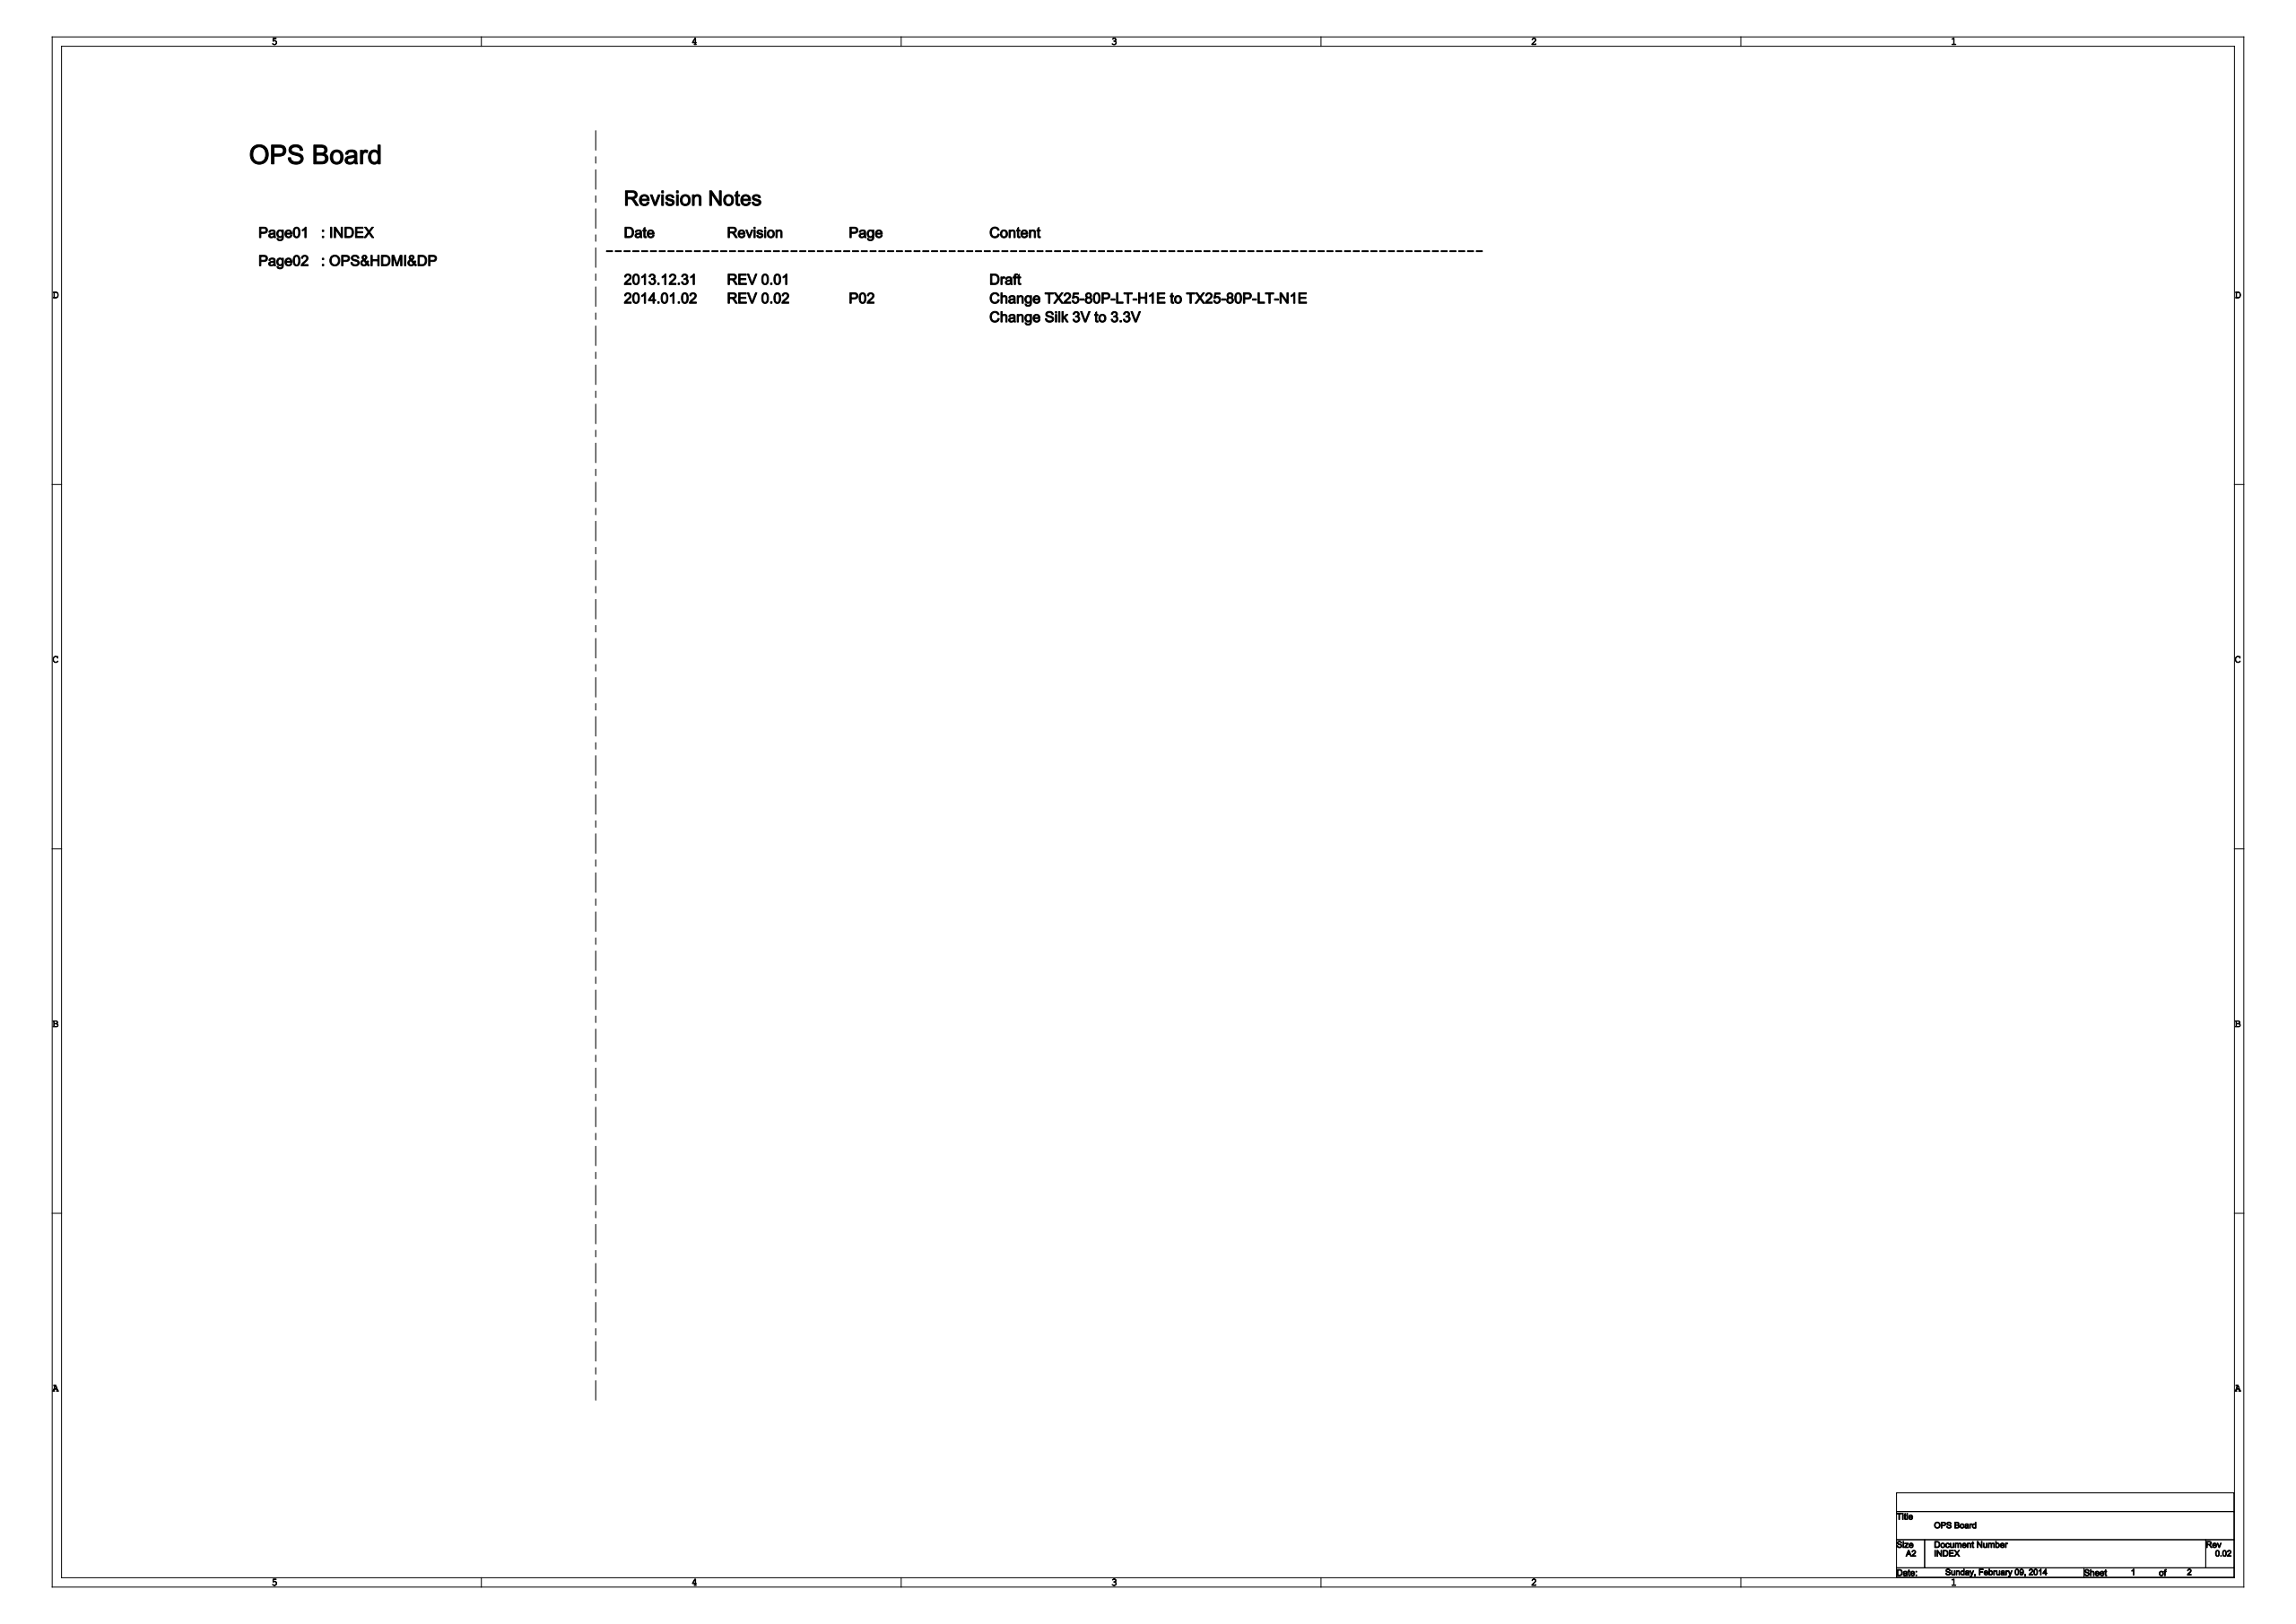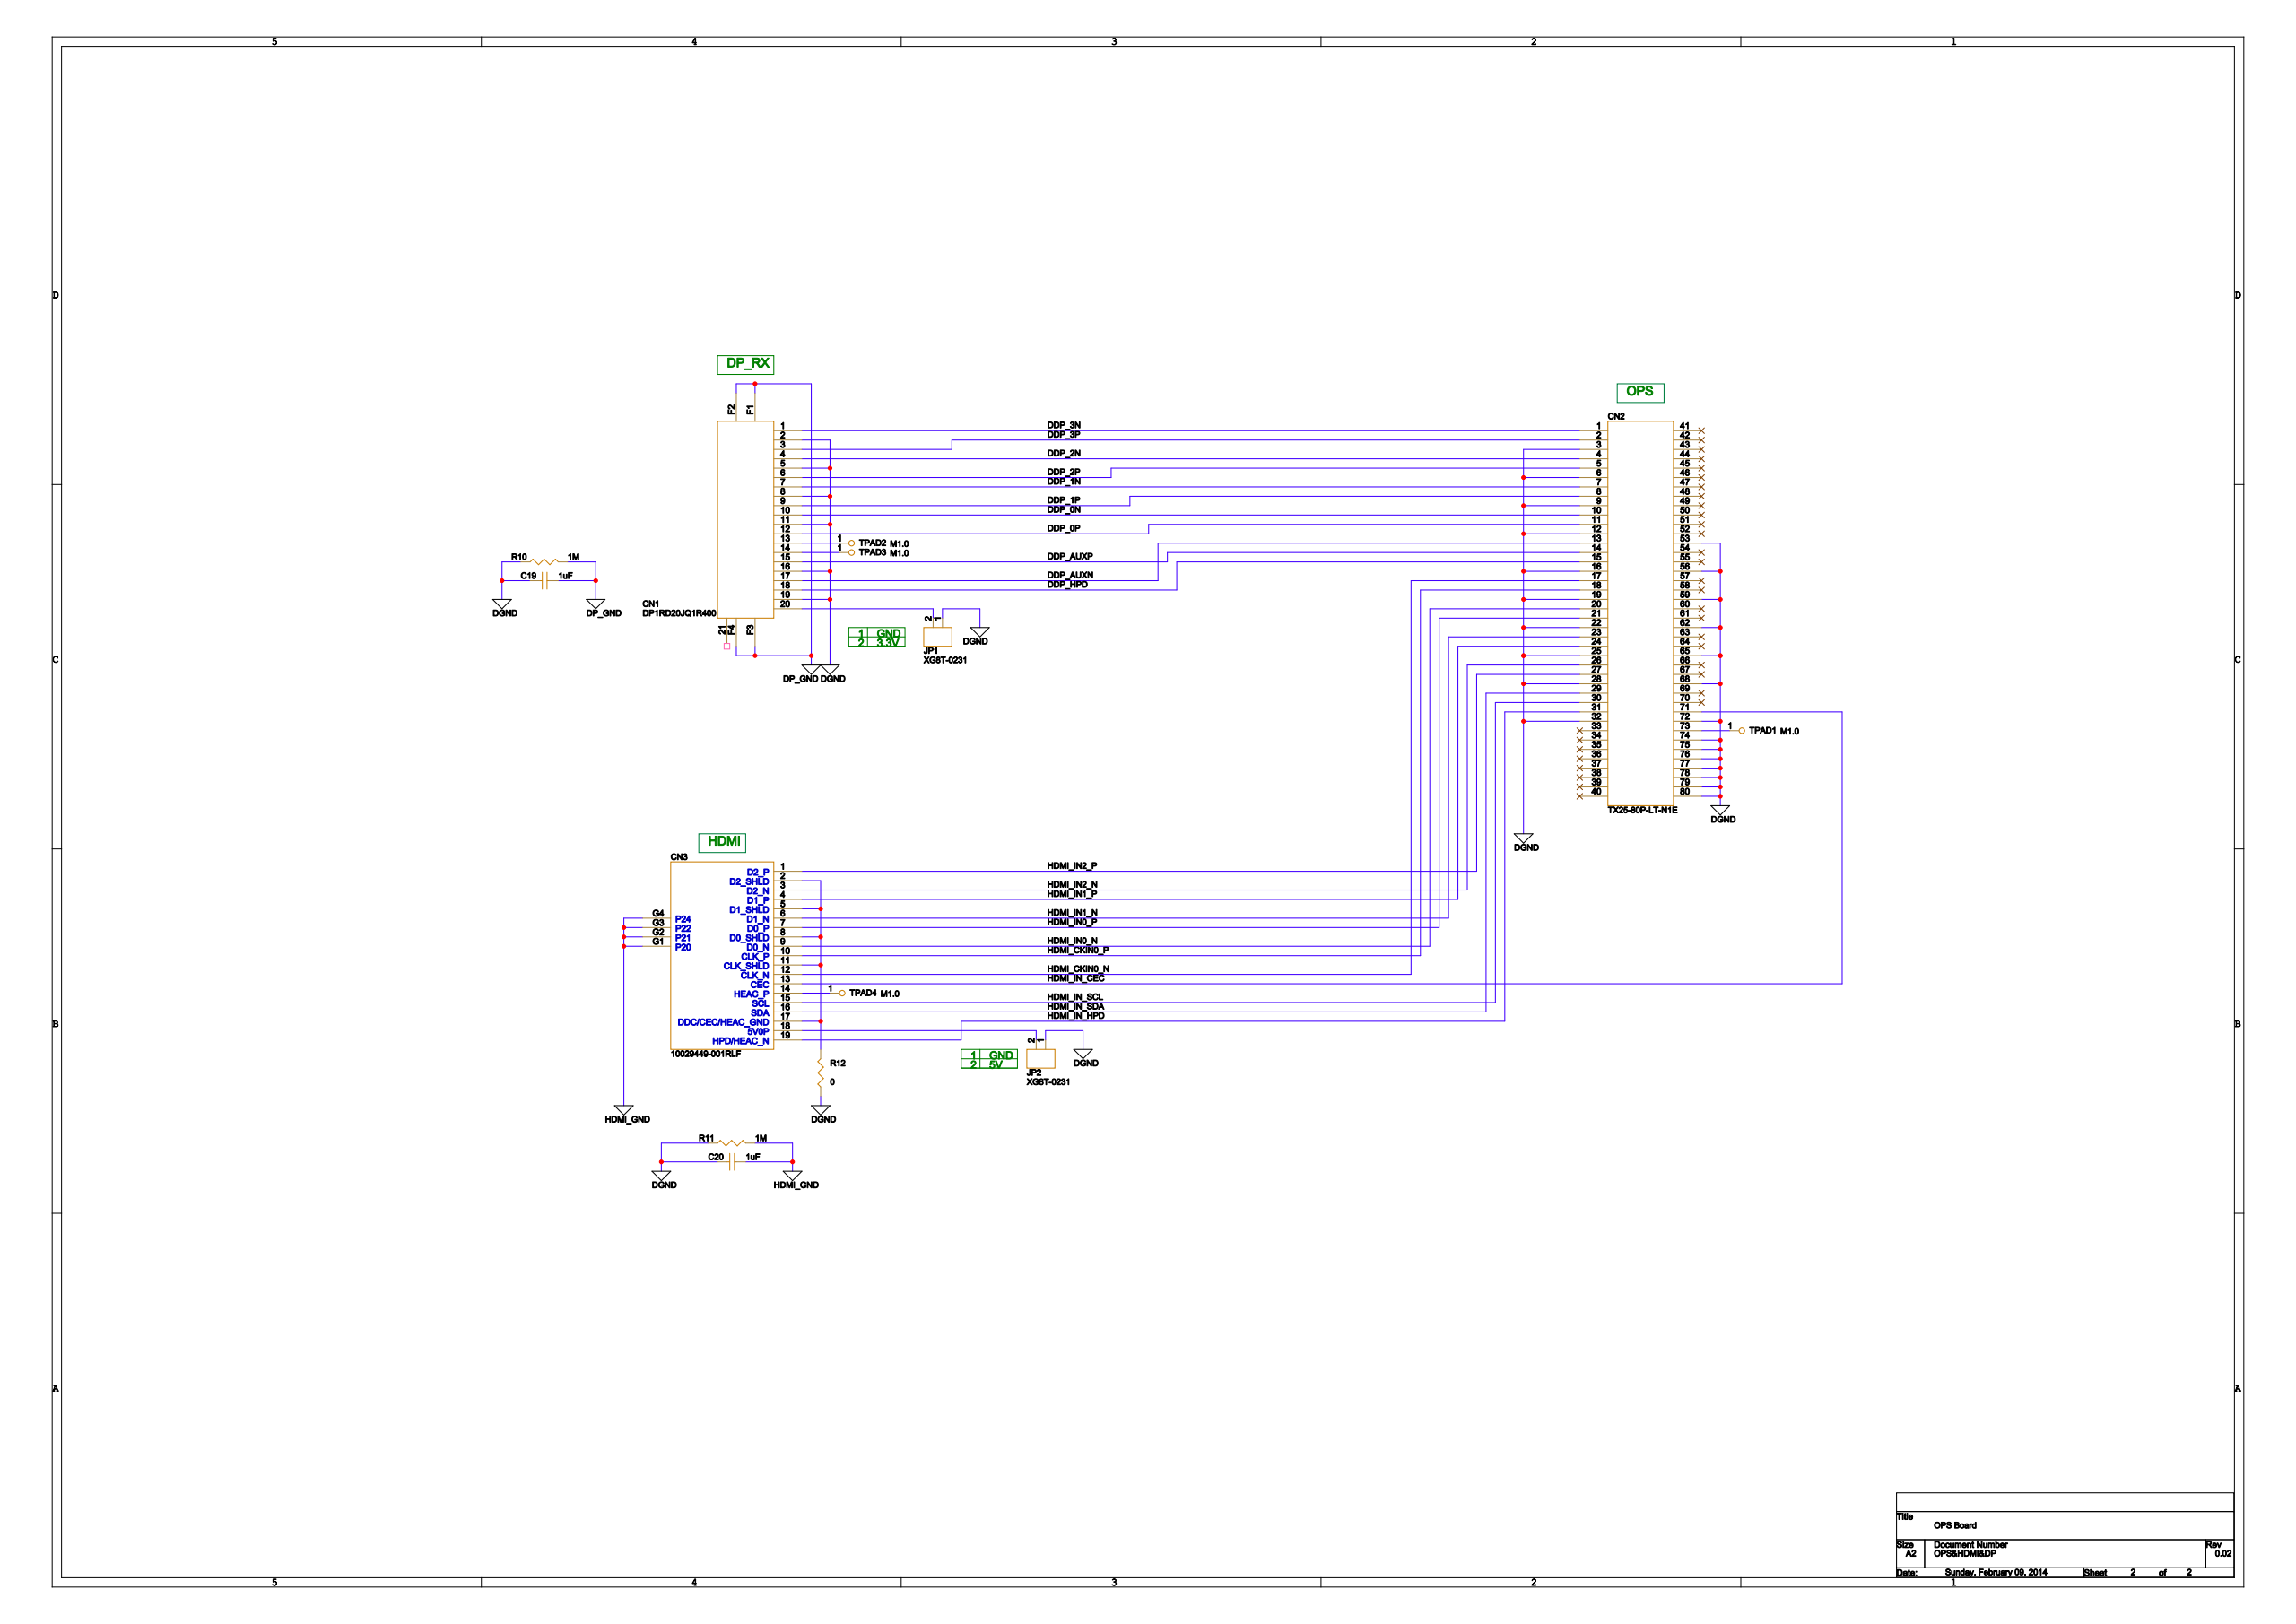Circuit board | Cadence Allegro | 14 parts | 33 nets
Bill of materials:
SYM_NAME,COMP_DEVICE_TYPE,COMP_VALUE,COMP_TOL,COMP_CLASS,REFDES
1005,CAPACITOR NON-POL_1005_1UF,1uF,,IC,C19
1005,CAPACITOR NON-POL_1005_1UF,1uF,,IC,C20
DP1RD20JQ1R400,DP1RD20JQ1R400_1_DP1RD20JQ1R400,DP1RD20JQ1R400,,IC,CN1
TX25-80P-LT-N1E,TX24-80R-LT-H1E_0_TX25-80P-LT-N,TX25-80P-LT-N1E,,IC,CN2
CON_HDMI_19F_20_SM_RA,HDMI_0_CON_HDMI_19F_20_SM_RA_10,10029449-001RLF,,IC,CN3
HDR1X2-2_54,CN3PIN_0_HDR1X2-2_54_XG8T-0231,XG8T-0231,,IC,JP1
HDR1X2-2_54,CN3PIN_0_HDR1X2-2_54_XG8T-0231,XG8T-0231,,IC,JP2
1608,R_1608_1M,1M,,IC,R10
1608,R_1608_1M,1M,,IC,R11
1608,R_1608_0,0,,IC,R12
TH_TC15-C10,TP-1_0_TH_TC15-C10_M1.0,M1.0,,IC,TPAD1
TH_TC15-C10,TP-1_0_TH_TC15-C10_M1.0,M1.0,,IC,TPAD2
TH_TC15-C10,TP-1_0_TH_TC15-C10_M1.0,M1.0,,IC,TPAD3
TH_TC15-C10,TP-1_0_TH_TC15-C10_M1.0,M1.0,,IC,TPAD4
Netlist (net: part-pin ...):
DDP_3N: CN1-1 CN2-1
DDP_0N: CN1-10 CN2-10
DGND: C19-2 C20-2 CN1-2 CN1-5 CN1-8 CN1-11 CN1-16 CN1-19 CN2-3 CN2-6 CN2-9 CN2-12 CN2-16 CN2-19 CN2-22 CN2-25 CN2-28 CN2-32 CN2-53 CN2-56 CN2-59 CN2-62 CN2-65 CN2-68 CN2-72 CN2-74 CN2-75 CN2-76 CN2-77 CN2-78 CN2-79 CN2-80 JP1-1 JP2-1 R10-1 R11-1 R12-1
DDP_0P: CN1-12 CN2-11
N16820349: CN1-13 TPAD2-1
N16820352: CN1-14 TPAD3-1
DDP_AUXP: CN1-15 CN2-14
DDP_AUXN: CN1-17 CN2-13
DDP_HPD: CN1-18 CN2-15
N16792414: CN1-20 JP1-2
DP_GND: C19-1 CN1-F1 CN1-F2 CN1-F3 CN1-F4 R10-2
DDP_3P: CN1-3 CN2-2
DDP_2N: CN1-4 CN2-4
DDP_2P: CN1-6 CN2-5
DDP_1N: CN1-7 CN2-7
DDP_1P: CN1-9 CN2-8
N16811230: CN3-18 JP2-2
HDMI_IN_CEC: CN2-71 CN3-13
HDMI_CKIN0_N: CN2-17 CN3-12
HDMI_CKIN0_P: CN2-18 CN3-10
N16813629: CN3-2 CN3-5 CN3-8 CN3-11 CN3-17 R12-2
HDMI_IN0_N: CN2-20 CN3-9
HDMI_IN0_P: CN2-21 CN3-7
HDMI_IN1_N: CN2-23 CN3-6
HDMI_IN1_P: CN2-24 CN3-4
HDMI_IN2_N: CN2-26 CN3-3
HDMI_IN2_P: CN2-27 CN3-1
N16820366: CN3-14 TPAD4-1
HDMI_IN_HPD: CN2-31 CN3-19
HDMI_GND: C20-1 CN3-G1 CN3-G2 CN3-G3 CN3-G4 R11-2
HDMI_IN_SCL: CN2-30 CN3-15
HDMI_IN_SDA: CN2-29 CN3-16
N16816227: CN2-73 TPAD1-1